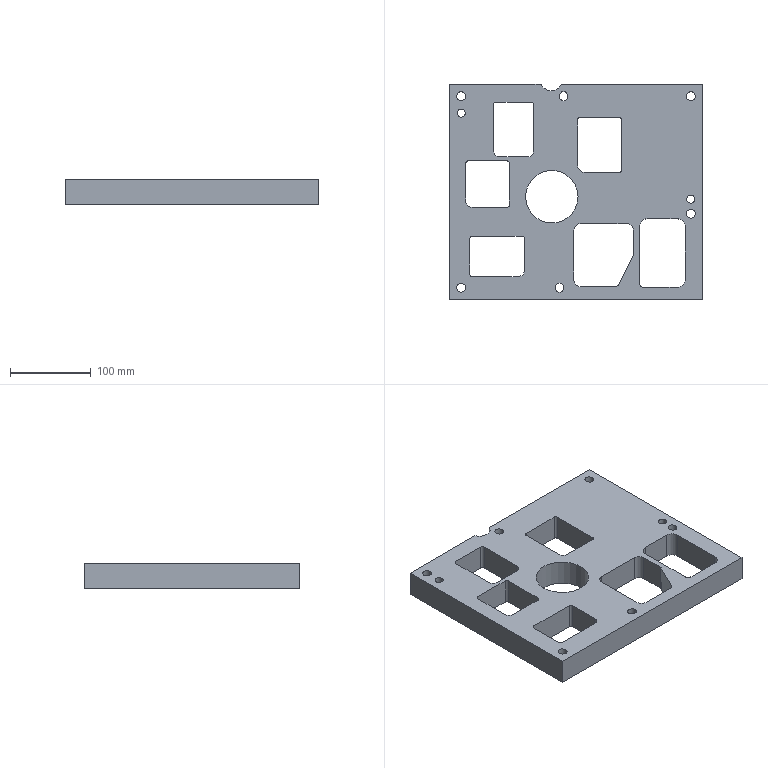Part | STEP file | lll_id3622_x_t | 1 solid | 83 faces | box 315 x 268 x 32 mm | volume 1792642 mm3 | cylinder 43 | plane 38 | cone 2 | commonest cylinder face diameters 6 x11 16 x8 11 x6 17 x6 10 x5 20 x3